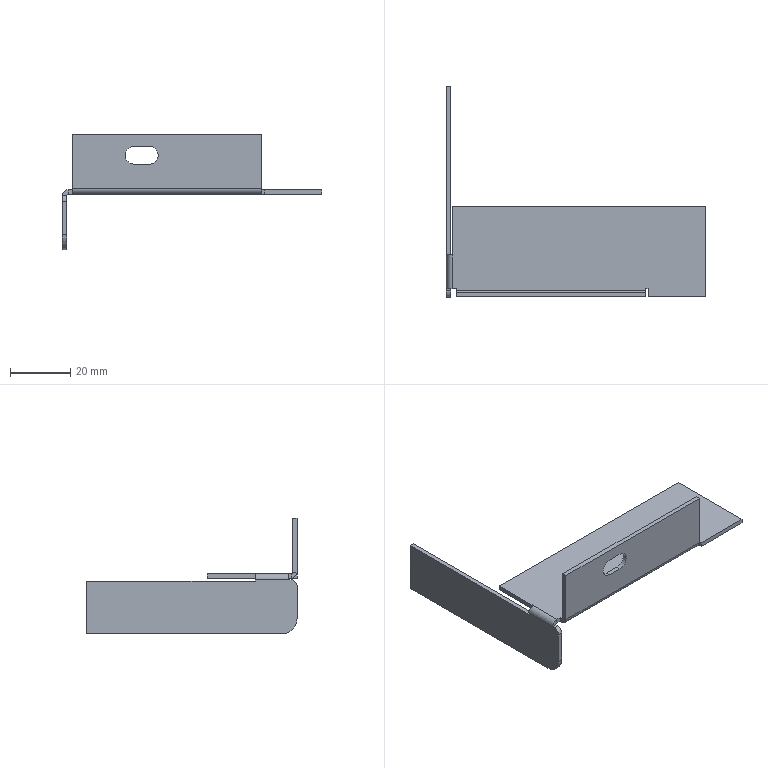Part | SolidWorks | features ICE 4, Fillet 2, EdgeFlange 1, FlatPattern 1, SMBaseFlange 1, SMMiteredFlange 1, SheetMetal 1 | 1 solid | 37 faces | box 86.5 x 70 x 38.5 mm | volume 7275 mm3 | plane 29 | cylinder 8 | commonest cylinder face diameters 4 x3 1 x2 6 x2 10 x1
STEP:
#1=CARTESIAN_POINT('',(-63.684,0.4966,0.));
#2=VERTEX_POINT('',#1);
#3=CARTESIAN_POINT('',(-63.684,-10.753,0.));
#4=VERTEX_POINT('',#3);
#5=CARTESIAN_POINT('',(-63.684,56.497,0.));
#6=DIRECTION('',(0.,-1.,0.));
#7=VECTOR('',#6,1000.);
#8=LINE('',#5,#7);
#9=EDGE_CURVE('',#2,#4,#8,.T.);
#10=ORIENTED_EDGE('',*,*,#9,.F.);
#11=CARTESIAN_POINT('',(-65.684,0.4966,-2.));
#12=VERTEX_POINT('',#11);
#13=CARTESIAN_POINT('',(-63.684,0.4966,-2.));
#14=DIRECTION('',(0.,-1.,0.));
#15=DIRECTION('',(0.,0.,1.));
#16=AXIS2_PLACEMENT_3D('',#13,#14,#15);
#17=CIRCLE('',#16,2.);
#18=EDGE_CURVE('',#2,#12,#17,.T.);
#19=ORIENTED_EDGE('',*,*,#18,.T.);
#20=CARTESIAN_POINT('',(-65.684,-10.753,-2.));
#21=VERTEX_POINT('',#20);
#22=CARTESIAN_POINT('',(-65.684,0.,-2.));
#23=DIRECTION('',(0.,1.,0.));
#24=VECTOR('',#23,1000.);
#25=LINE('',#22,#24);
#26=EDGE_CURVE('',#21,#12,#25,.T.);
#27=ORIENTED_EDGE('',*,*,#26,.F.);
#28=CARTESIAN_POINT('',(-63.684,-10.753,-2.));
#29=DIRECTION('',(0.,-1.,0.));
#30=DIRECTION('',(0.,0.,1.));
#31=AXIS2_PLACEMENT_3D('',#28,#29,#30);
#32=CIRCLE('',#31,2.);
#33=EDGE_CURVE('',#4,#21,#32,.T.);
#34=ORIENTED_EDGE('',*,*,#33,.F.);
#35=EDGE_LOOP('',(#10,#19,#27,#34));
#36=FACE_OUTER_BOUND('',#35,.T.);
#37=CARTESIAN_POINT('',(-63.684,56.497,-2.));
#38=DIRECTION('',(0.,1.,0.));
#39=DIRECTION('',(-1.,0.,0.));
#40=AXIS2_PLACEMENT_3D('',#37,#38,#39);
#41=CYLINDRICAL_SURFACE('',#40,2.);
#42=ADVANCED_FACE('',(#36),#41,.T.);
#43=CARTESIAN_POINT('',(-63.684,0.4966,-1.5));
#44=VERTEX_POINT('',#43);
#45=CARTESIAN_POINT('',(-64.184,0.4966,-2.));
#46=VERTEX_POINT('',#45);
#47=CARTESIAN_POINT('',(-63.684,0.4966,-2.));
#48=DIRECTION('',(0.,-1.,0.));
#49=DIRECTION('',(0.,0.,1.));
#50=AXIS2_PLACEMENT_3D('',#47,#48,#49);
#51=CIRCLE('',#50,0.5);
#52=EDGE_CURVE('',#44,#46,#51,.T.);
#53=ORIENTED_EDGE('',*,*,#52,.F.);
#54=CARTESIAN_POINT('',(-63.684,-10.753,-1.5));
#55=VERTEX_POINT('',#54);
#56=CARTESIAN_POINT('',(-63.684,56.497,-1.5));
#57=DIRECTION('',(0.,-1.,0.));
#58=VECTOR('',#57,1000.);
#59=LINE('',#56,#58);
#60=EDGE_CURVE('',#44,#55,#59,.T.);
#61=ORIENTED_EDGE('',*,*,#60,.T.);
#62=CARTESIAN_POINT('',(-64.184,-10.753,-2.));
#63=VERTEX_POINT('',#62);
#64=CARTESIAN_POINT('',(-63.684,-10.753,-2.));
#65=DIRECTION('',(0.,-1.,0.));
#66=DIRECTION('',(0.,0.,1.));
#67=AXIS2_PLACEMENT_3D('',#64,#65,#66);
#68=CIRCLE('',#67,0.5);
#69=EDGE_CURVE('',#55,#63,#68,.T.);
#70=ORIENTED_EDGE('',*,*,#69,.T.);
#71=CARTESIAN_POINT('',(-64.184,-13.503,-2.));
#72=DIRECTION('',(0.,1.,0.));
#73=VECTOR('',#72,1000.);
#74=LINE('',#71,#73);
#75=EDGE_CURVE('',#63,#46,#74,.T.);
#76=ORIENTED_EDGE('',*,*,#75,.T.);
#77=EDGE_LOOP('',(#53,#61,#70,#76));
#78=FACE_OUTER_BOUND('',#77,.T.);
#79=CARTESIAN_POINT('',(-63.684,56.497,-2.));
#80=DIRECTION('',(0.,1.,0.));
#81=DIRECTION('',(-1.,0.,0.));
#82=AXIS2_PLACEMENT_3D('',#79,#80,#81);
#83=CYLINDRICAL_SURFACE('',#82,0.5);
#84=ADVANCED_FACE('',(#78),#83,.F.);
#85=CARTESIAN_POINT('',(-62.184,-10.753,-1.5));
#86=VERTEX_POINT('',#85);
#87=CARTESIAN_POINT('',(-62.184,-10.753,-1.5));
#88=DIRECTION('',(-1.,0.,0.));
#89=VECTOR('',#88,1000.);
#90=LINE('',#87,#89);
#91=EDGE_CURVE('',#86,#55,#90,.T.);
#92=ORIENTED_EDGE('',*,*,#91,.T.);
#93=ORIENTED_EDGE('',*,*,#60,.F.);
#94=CARTESIAN_POINT('',(-63.684,16.497,-1.5));
#95=VERTEX_POINT('',#94);
#96=CARTESIAN_POINT('',(-63.684,56.497,-1.5));
#97=DIRECTION('',(0.,-1.,0.));
#98=VECTOR('',#97,1000.);
#99=LINE('',#96,#98);
#100=EDGE_CURVE('',#95,#44,#99,.T.);
#101=ORIENTED_EDGE('',*,*,#100,.F.);
#102=CARTESIAN_POINT('',(20.816,16.497,-1.5));
#103=VERTEX_POINT('',#102);
#104=CARTESIAN_POINT('',(0.,16.497,-1.5));
#105=DIRECTION('',(1.,0.,0.));
#106=VECTOR('',#105,1000.);
#107=LINE('',#104,#106);
#108=EDGE_CURVE('',#95,#103,#107,.T.);
#109=ORIENTED_EDGE('',*,*,#108,.T.);
#110=CARTESIAN_POINT('',(20.816,-13.503,-1.5));
#111=VERTEX_POINT('',#110);
#112=CARTESIAN_POINT('',(20.816,70.497,-1.5));
#113=DIRECTION('',(0.,1.,0.));
#114=VECTOR('',#113,1000.);
#115=LINE('',#112,#114);
#116=EDGE_CURVE('',#111,#103,#115,.T.);
#117=ORIENTED_EDGE('',*,*,#116,.F.);
#118=CARTESIAN_POINT('',(1.566,-13.503,-1.5));
#119=VERTEX_POINT('',#118);
#120=CARTESIAN_POINT('',(-64.184,-13.503,-1.5));
#121=DIRECTION('',(1.,0.,0.));
#122=VECTOR('',#121,1000.);
#123=LINE('',#120,#122);
#124=EDGE_CURVE('',#119,#111,#123,.T.);
#125=ORIENTED_EDGE('',*,*,#124,.F.);
#126=CARTESIAN_POINT('',(1.566,-10.753,-1.5));
#127=VERTEX_POINT('',#126);
#128=CARTESIAN_POINT('',(1.566,-10.753,-1.5));
#129=DIRECTION('',(0.,-1.,0.));
#130=VECTOR('',#129,1000.);
#131=LINE('',#128,#130);
#132=EDGE_CURVE('',#127,#119,#131,.T.);
#133=ORIENTED_EDGE('',*,*,#132,.F.);
#134=CARTESIAN_POINT('',(0.8165,-10.753,-1.5));
#135=VERTEX_POINT('',#134);
#136=CARTESIAN_POINT('',(0.8165,-10.753,-1.5));
#137=DIRECTION('',(1.,0.,0.));
#138=VECTOR('',#137,1000.);
#139=LINE('',#136,#138);
#140=EDGE_CURVE('',#135,#127,#139,.T.);
#141=ORIENTED_EDGE('',*,*,#140,.F.);
#142=CARTESIAN_POINT('',(0.8165,-11.503,-1.5));
#143=VERTEX_POINT('',#142);
#144=CARTESIAN_POINT('',(0.8165,-13.503,-1.5));
#145=DIRECTION('',(0.,1.,0.));
#146=VECTOR('',#145,1000.);
#147=LINE('',#144,#146);
#148=EDGE_CURVE('',#143,#135,#147,.T.);
#149=ORIENTED_EDGE('',*,*,#148,.F.);
#150=CARTESIAN_POINT('',(-62.184,-11.503,-1.5));
#151=VERTEX_POINT('',#150);
#152=CARTESIAN_POINT('',(445.816,-11.503,-1.5));
#153=DIRECTION('',(-1.,0.,0.));
#154=VECTOR('',#153,1000.);
#155=LINE('',#152,#154);
#156=EDGE_CURVE('',#143,#151,#155,.T.);
#157=ORIENTED_EDGE('',*,*,#156,.T.);
#158=CARTESIAN_POINT('',(-62.184,-13.503,-1.5));
#159=DIRECTION('',(0.,1.,0.));
#160=VECTOR('',#159,1000.);
#161=LINE('',#158,#160);
#162=EDGE_CURVE('',#151,#86,#161,.T.);
#163=ORIENTED_EDGE('',*,*,#162,.T.);
#164=EDGE_LOOP('',(#92,#93,#101,#109,#117,#125,#133,#141,#149,#157,#163));
#165=FACE_OUTER_BOUND('',#164,.T.);
#166=CARTESIAN_POINT('',(0.,0.,-1.5));
#167=DIRECTION('',(0.,0.,1.));
#168=DIRECTION('',(1.,0.,0.));
#169=AXIS2_PLACEMENT_3D('',#166,#167,#168);
#170=PLANE('',#169);
#171=ADVANCED_FACE('',(#165),#170,.F.);
#172=CARTESIAN_POINT('',(-63.684,16.497,0.));
#173=VERTEX_POINT('',#172);
#174=CARTESIAN_POINT('',(-63.684,56.497,0.));
#175=DIRECTION('',(0.,-1.,0.));
#176=VECTOR('',#175,1000.);
#177=LINE('',#174,#176);
#178=EDGE_CURVE('',#173,#2,#177,.T.);
#179=ORIENTED_EDGE('',*,*,#178,.T.);
#180=ORIENTED_EDGE('',*,*,#9,.T.);
#181=CARTESIAN_POINT('',(-62.184,-10.753,0.));
#182=VERTEX_POINT('',#181);
#183=CARTESIAN_POINT('',(-62.184,-10.753,0.));
#184=DIRECTION('',(-1.,0.,0.));
#185=VECTOR('',#184,1000.);
#186=LINE('',#183,#185);
#187=EDGE_CURVE('',#182,#4,#186,.T.);
#188=ORIENTED_EDGE('',*,*,#187,.F.);
#189=CARTESIAN_POINT('',(-62.184,-11.503,0.));
#190=VERTEX_POINT('',#189);
#191=CARTESIAN_POINT('',(-62.184,-13.503,0.));
#192=DIRECTION('',(0.,1.,0.));
#193=VECTOR('',#192,1000.);
#194=LINE('',#191,#193);
#195=EDGE_CURVE('',#190,#182,#194,.T.);
#196=ORIENTED_EDGE('',*,*,#195,.F.);
#197=CARTESIAN_POINT('',(0.8165,-11.503,0.));
#198=VERTEX_POINT('',#197);
#199=CARTESIAN_POINT('',(445.816,-11.503,0.));
#200=DIRECTION('',(-1.,0.,0.));
#201=VECTOR('',#200,1000.);
#202=LINE('',#199,#201);
#203=EDGE_CURVE('',#198,#190,#202,.T.);
#204=ORIENTED_EDGE('',*,*,#203,.F.);
#205=CARTESIAN_POINT('',(0.8165,-10.753,0.));
#206=VERTEX_POINT('',#205);
#207=CARTESIAN_POINT('',(0.8165,-13.503,0.));
#208=DIRECTION('',(0.,1.,0.));
#209=VECTOR('',#208,1000.);
#210=LINE('',#207,#209);
#211=EDGE_CURVE('',#198,#206,#210,.T.);
#212=ORIENTED_EDGE('',*,*,#211,.T.);
#213=CARTESIAN_POINT('',(1.566,-10.753,0.));
#214=VERTEX_POINT('',#213);
#215=CARTESIAN_POINT('',(0.8165,-10.753,0.));
#216=DIRECTION('',(1.,0.,0.));
#217=VECTOR('',#216,1000.);
#218=LINE('',#215,#217);
#219=EDGE_CURVE('',#206,#214,#218,.T.);
#220=ORIENTED_EDGE('',*,*,#219,.T.);
#221=CARTESIAN_POINT('',(1.566,-13.503,0.));
#222=VERTEX_POINT('',#221);
#223=CARTESIAN_POINT('',(1.566,-10.753,0.));
#224=DIRECTION('',(0.,-1.,0.));
#225=VECTOR('',#224,1000.);
#226=LINE('',#223,#225);
#227=EDGE_CURVE('',#214,#222,#226,.T.);
#228=ORIENTED_EDGE('',*,*,#227,.T.);
#229=CARTESIAN_POINT('',(20.816,-13.503,0.));
#230=VERTEX_POINT('',#229);
#231=CARTESIAN_POINT('',(-64.184,-13.503,0.));
#232=DIRECTION('',(1.,0.,0.));
#233=VECTOR('',#232,1000.);
#234=LINE('',#231,#233);
#235=EDGE_CURVE('',#222,#230,#234,.T.);
#236=ORIENTED_EDGE('',*,*,#235,.T.);
#237=CARTESIAN_POINT('',(20.816,16.497,0.));
#238=VERTEX_POINT('',#237);
#239=CARTESIAN_POINT('',(20.816,70.497,0.));
#240=DIRECTION('',(0.,1.,0.));
#241=VECTOR('',#240,1000.);
#242=LINE('',#239,#241);
#243=EDGE_CURVE('',#230,#238,#242,.T.);
#244=ORIENTED_EDGE('',*,*,#243,.T.);
#245=CARTESIAN_POINT('',(0.,16.497,0.));
#246=DIRECTION('',(1.,0.,0.));
#247=VECTOR('',#246,1000.);
#248=LINE('',#245,#247);
#249=EDGE_CURVE('',#173,#238,#248,.T.);
#250=ORIENTED_EDGE('',*,*,#249,.F.);
#251=EDGE_LOOP('',(#179,#180,#188,#196,#204,#212,#220,#228,#236,#244,#250));
#252=FACE_OUTER_BOUND('',#251,.T.);
#253=CARTESIAN_POINT('',(0.,0.,0.));
#254=DIRECTION('',(0.,0.,1.));
#255=DIRECTION('',(1.,0.,0.));
#256=AXIS2_PLACEMENT_3D('',#253,#254,#255);
#257=PLANE('',#256);
#258=ADVANCED_FACE('',(#252),#257,.T.);
#259=ORIENTED_EDGE('',*,*,#116,.T.);
#260=CARTESIAN_POINT('',(20.816,16.497,-1.5));
#261=DIRECTION('',(0.,0.,1.));
#262=VECTOR('',#261,1000.);
#263=LINE('',#260,#262);
#264=EDGE_CURVE('',#103,#238,#263,.T.);
#265=ORIENTED_EDGE('',*,*,#264,.T.);
#266=ORIENTED_EDGE('',*,*,#243,.F.);
#267=CARTESIAN_POINT('',(20.816,-13.503,-1.5));
#268=DIRECTION('',(0.,0.,1.));
#269=VECTOR('',#268,1000.);
#270=LINE('',#267,#269);
#271=EDGE_CURVE('',#111,#230,#270,.T.);
#272=ORIENTED_EDGE('',*,*,#271,.F.);
#273=EDGE_LOOP('',(#259,#265,#266,#272));
#274=FACE_OUTER_BOUND('',#273,.T.);
#275=CARTESIAN_POINT('',(20.816,70.497,-1.5));
#276=DIRECTION('',(1.,0.,0.));
#277=DIRECTION('',(0.,1.,0.));
#278=AXIS2_PLACEMENT_3D('',#275,#276,#277);
#279=PLANE('',#278);
#280=ADVANCED_FACE('',(#274),#279,.T.);
#281=CARTESIAN_POINT('',(1.566,-13.503,0.));
#282=DIRECTION('',(0.,0.,-1.));
#283=VECTOR('',#282,1000.);
#284=LINE('',#281,#283);
#285=EDGE_CURVE('',#222,#119,#284,.T.);
#286=ORIENTED_EDGE('',*,*,#285,.T.);
#287=ORIENTED_EDGE('',*,*,#124,.T.);
#288=ORIENTED_EDGE('',*,*,#271,.T.);
#289=ORIENTED_EDGE('',*,*,#235,.F.);
#290=EDGE_LOOP('',(#286,#287,#288,#289));
#291=FACE_OUTER_BOUND('',#290,.T.);
#292=CARTESIAN_POINT('',(-64.184,-13.503,-1.5));
#293=DIRECTION('',(0.,-1.,0.));
#294=DIRECTION('',(0.,0.,-1.));
#295=AXIS2_PLACEMENT_3D('',#292,#293,#294);
#296=PLANE('',#295);
#297=ADVANCED_FACE('',(#291),#296,.T.);
#298=CARTESIAN_POINT('',(0.8165,-11.503,-1.5));
#299=DIRECTION('',(0.,0.,1.));
#300=VECTOR('',#299,1000.);
#301=LINE('',#298,#300);
#302=EDGE_CURVE('',#143,#198,#301,.T.);
#303=ORIENTED_EDGE('',*,*,#302,.F.);
#304=ORIENTED_EDGE('',*,*,#148,.T.);
#305=CARTESIAN_POINT('',(0.8165,-10.753,0.));
#306=DIRECTION('',(0.,0.,-1.));
#307=VECTOR('',#306,1000.);
#308=LINE('',#305,#307);
#309=EDGE_CURVE('',#206,#135,#308,.T.);
#310=ORIENTED_EDGE('',*,*,#309,.F.);
#311=ORIENTED_EDGE('',*,*,#211,.F.);
#312=EDGE_LOOP('',(#303,#304,#310,#311));
#313=FACE_OUTER_BOUND('',#312,.T.);
#314=CARTESIAN_POINT('',(0.8165,-13.503,0.));
#315=DIRECTION('',(-1.,0.,0.));
#316=DIRECTION('',(0.,0.,1.));
#317=AXIS2_PLACEMENT_3D('',#314,#315,#316);
#318=PLANE('',#317);
#319=ADVANCED_FACE('',(#313),#318,.F.);
#320=ORIENTED_EDGE('',*,*,#140,.T.);
#321=CARTESIAN_POINT('',(1.566,-10.753,0.));
#322=DIRECTION('',(0.,0.,-1.));
#323=VECTOR('',#322,1000.);
#324=LINE('',#321,#323);
#325=EDGE_CURVE('',#214,#127,#324,.T.);
#326=ORIENTED_EDGE('',*,*,#325,.F.);
#327=ORIENTED_EDGE('',*,*,#219,.F.);
#328=ORIENTED_EDGE('',*,*,#309,.T.);
#329=EDGE_LOOP('',(#320,#326,#327,#328));
#330=FACE_OUTER_BOUND('',#329,.T.);
#331=CARTESIAN_POINT('',(0.8165,-10.753,0.));
#332=DIRECTION('',(0.,1.,0.));
#333=DIRECTION('',(0.,0.,1.));
#334=AXIS2_PLACEMENT_3D('',#331,#332,#333);
#335=PLANE('',#334);
#336=ADVANCED_FACE('',(#330),#335,.F.);
#337=ORIENTED_EDGE('',*,*,#132,.T.);
#338=ORIENTED_EDGE('',*,*,#285,.F.);
#339=ORIENTED_EDGE('',*,*,#227,.F.);
#340=ORIENTED_EDGE('',*,*,#325,.T.);
#341=EDGE_LOOP('',(#337,#338,#339,#340));
#342=FACE_OUTER_BOUND('',#341,.T.);
#343=CARTESIAN_POINT('',(1.566,-10.753,0.));
#344=DIRECTION('',(1.,0.,0.));
#345=DIRECTION('',(0.,0.,-1.));
#346=AXIS2_PLACEMENT_3D('',#343,#344,#345);
#347=PLANE('',#346);
#348=ADVANCED_FACE('',(#342),#347,.F.);
#349=ORIENTED_EDGE('',*,*,#195,.T.);
#350=CARTESIAN_POINT('',(-62.184,-10.753,0.));
#351=DIRECTION('',(0.,0.,-1.));
#352=VECTOR('',#351,1000.);
#353=LINE('',#350,#352);
#354=EDGE_CURVE('',#182,#86,#353,.T.);
#355=ORIENTED_EDGE('',*,*,#354,.T.);
#356=ORIENTED_EDGE('',*,*,#162,.F.);
#357=CARTESIAN_POINT('',(-62.184,-11.503,-1.5));
#358=DIRECTION('',(0.,0.,1.));
#359=VECTOR('',#358,1000.);
#360=LINE('',#357,#359);
#361=EDGE_CURVE('',#151,#190,#360,.T.);
#362=ORIENTED_EDGE('',*,*,#361,.T.);
#363=EDGE_LOOP('',(#349,#355,#356,#362));
#364=FACE_OUTER_BOUND('',#363,.T.);
#365=CARTESIAN_POINT('',(-62.184,-13.503,0.));
#366=DIRECTION('',(-1.,0.,0.));
#367=DIRECTION('',(0.,0.,1.));
#368=AXIS2_PLACEMENT_3D('',#365,#366,#367);
#369=PLANE('',#368);
#370=ADVANCED_FACE('',(#364),#369,.T.);
#371=ORIENTED_EDGE('',*,*,#91,.F.);
#372=ORIENTED_EDGE('',*,*,#354,.F.);
#373=ORIENTED_EDGE('',*,*,#187,.T.);
#374=CARTESIAN_POINT('',(-63.684,-10.753,0.));
#375=DIRECTION('',(0.,0.,-1.));
#376=VECTOR('',#375,1000.);
#377=LINE('',#374,#376);
#378=EDGE_CURVE('',#4,#55,#377,.T.);
#379=ORIENTED_EDGE('',*,*,#378,.T.);
#380=EDGE_LOOP('',(#371,#372,#373,#379));
#381=FACE_OUTER_BOUND('',#380,.T.);
#382=CARTESIAN_POINT('',(-62.184,-10.753,0.));
#383=DIRECTION('',(0.,-1.,0.));
#384=DIRECTION('',(0.,0.,-1.));
#385=AXIS2_PLACEMENT_3D('',#382,#383,#384);
#386=PLANE('',#385);
#387=ADVANCED_FACE('',(#381),#386,.T.);
#388=CARTESIAN_POINT('',(-62.184,-13.503,18.5));
#389=VERTEX_POINT('',#388);
#390=CARTESIAN_POINT('',(-62.184,-12.003,18.5));
#391=VERTEX_POINT('',#390);
#392=CARTESIAN_POINT('',(-62.184,-13.503,18.5));
#393=DIRECTION('',(0.,1.,0.));
#394=VECTOR('',#393,1000.);
#395=LINE('',#392,#394);
#396=EDGE_CURVE('',#389,#391,#395,.T.);
#397=ORIENTED_EDGE('',*,*,#396,.F.);
#398=CARTESIAN_POINT('',(0.8165,-13.503,18.5));
#399=VERTEX_POINT('',#398);
#400=CARTESIAN_POINT('',(20.816,-13.503,18.5));
#401=DIRECTION('',(-1.,0.,0.));
#402=VECTOR('',#401,1000.);
#403=LINE('',#400,#402);
#404=EDGE_CURVE('',#399,#389,#403,.T.);
#405=ORIENTED_EDGE('',*,*,#404,.F.);
#406=CARTESIAN_POINT('',(0.8165,-12.003,18.5));
#407=VERTEX_POINT('',#406);
#408=CARTESIAN_POINT('',(0.8165,-13.503,18.5));
#409=DIRECTION('',(0.,1.,0.));
#410=VECTOR('',#409,1000.);
#411=LINE('',#408,#410);
#412=EDGE_CURVE('',#399,#407,#411,.T.);
#413=ORIENTED_EDGE('',*,*,#412,.T.);
#414=CARTESIAN_POINT('',(20.816,-12.003,18.5));
#415=DIRECTION('',(-1.,0.,0.));
#416=VECTOR('',#415,1000.);
#417=LINE('',#414,#416);
#418=EDGE_CURVE('',#407,#391,#417,.T.);
#419=ORIENTED_EDGE('',*,*,#418,.T.);
#420=EDGE_LOOP('',(#397,#405,#413,#419));
#421=FACE_OUTER_BOUND('',#420,.T.);
#422=CARTESIAN_POINT('',(20.816,-13.503,18.5));
#423=DIRECTION('',(0.,0.,-1.));
#424=DIRECTION('',(-1.,0.,0.));
#425=AXIS2_PLACEMENT_3D('',#422,#423,#424);
#426=PLANE('',#425);
#427=ADVANCED_FACE('',(#421),#426,.F.);
#428=ORIENTED_EDGE('',*,*,#412,.F.);
#429=CARTESIAN_POINT('',(0.8165,-13.503,0.5));
#430=VERTEX_POINT('',#429);
#431=CARTESIAN_POINT('',(0.8165,-13.503,18.5));
#432=DIRECTION('',(0.,0.,-1.));
#433=VECTOR('',#432,1000.);
#434=LINE('',#431,#433);
#435=EDGE_CURVE('',#399,#430,#434,.T.);
#436=ORIENTED_EDGE('',*,*,#435,.T.);
#437=CARTESIAN_POINT('',(0.8165,-12.003,0.5));
#438=VERTEX_POINT('',#437);
#439=CARTESIAN_POINT('',(0.8165,-13.503,0.5));
#440=DIRECTION('',(0.,1.,0.));
#441=VECTOR('',#440,1000.);
#442=LINE('',#439,#441);
#443=EDGE_CURVE('',#430,#438,#442,.T.);
#444=ORIENTED_EDGE('',*,*,#443,.T.);
#445=CARTESIAN_POINT('',(0.8165,-12.003,18.5));
#446=DIRECTION('',(0.,0.,-1.));
#447=VECTOR('',#446,1000.);
#448=LINE('',#445,#447);
#449=EDGE_CURVE('',#407,#438,#448,.T.);
#450=ORIENTED_EDGE('',*,*,#449,.F.);
#451=EDGE_LOOP('',(#428,#436,#444,#450));
#452=FACE_OUTER_BOUND('',#451,.T.);
#453=CARTESIAN_POINT('',(0.8165,-13.503,18.5));
#454=DIRECTION('',(1.,0.,0.));
#455=DIRECTION('',(0.,0.,-1.));
#456=AXIS2_PLACEMENT_3D('',#453,#454,#455);
#457=PLANE('',#456);
#458=ADVANCED_FACE('',(#452),#457,.T.);
#459=CARTESIAN_POINT('',(-62.184,-13.503,0.5));
#460=VERTEX_POINT('',#459);
#461=CARTESIAN_POINT('',(-62.184,-13.503,18.5));
#462=DIRECTION('',(0.,0.,1.));
#463=VECTOR('',#462,1000.);
#464=LINE('',#461,#463);
#465=EDGE_CURVE('',#460,#389,#464,.T.);
#466=ORIENTED_EDGE('',*,*,#465,.T.);
#467=ORIENTED_EDGE('',*,*,#396,.T.);
#468=CARTESIAN_POINT('',(-62.184,-12.003,0.5));
#469=VERTEX_POINT('',#468);
#470=CARTESIAN_POINT('',(-62.184,-12.003,18.5));
#471=DIRECTION('',(0.,0.,1.));
#472=VECTOR('',#471,1000.);
#473=LINE('',#470,#472);
#474=EDGE_CURVE('',#469,#391,#473,.T.);
#475=ORIENTED_EDGE('',*,*,#474,.F.);
#476=CARTESIAN_POINT('',(-62.184,-13.503,0.5));
#477=DIRECTION('',(0.,1.,0.));
#478=VECTOR('',#477,1000.);
#479=LINE('',#476,#478);
#480=EDGE_CURVE('',#460,#469,#479,.T.);
#481=ORIENTED_EDGE('',*,*,#480,.F.);
#482=EDGE_LOOP('',(#466,#467,#475,#481));
#483=FACE_OUTER_BOUND('',#482,.T.);
#484=CARTESIAN_POINT('',(-62.184,-13.503,18.5));
#485=DIRECTION('',(-1.,0.,0.));
#486=DIRECTION('',(0.,0.,1.));
#487=AXIS2_PLACEMENT_3D('',#484,#485,#486);
#488=PLANE('',#487);
#489=ADVANCED_FACE('',(#483),#488,.T.);
#490=CARTESIAN_POINT('',(-41.684,-12.003,8.5));
#491=VERTEX_POINT('',#490);
#492=CARTESIAN_POINT('',(-41.684,-12.003,14.5));
#493=VERTEX_POINT('',#492);
#494=CARTESIAN_POINT('',(-41.684,-12.003,11.5));
#495=DIRECTION('',(0.,1.,0.));
#496=DIRECTION('',(0.,0.,1.));
#497=AXIS2_PLACEMENT_3D('',#494,#495,#496);
#498=CIRCLE('',#497,3.);
#499=EDGE_CURVE('',#491,#493,#498,.T.);
#500=ORIENTED_EDGE('',*,*,#499,.F.);
#501=CARTESIAN_POINT('',(-36.684,-12.003,8.5));
#502=VERTEX_POINT('',#501);
#503=CARTESIAN_POINT('',(-41.684,-12.003,8.5));
#504=DIRECTION('',(-1.,0.,0.));
#505=VECTOR('',#504,1000.);
#506=LINE('',#503,#505);
#507=EDGE_CURVE('',#502,#491,#506,.T.);
#508=ORIENTED_EDGE('',*,*,#507,.F.);
#509=CARTESIAN_POINT('',(-36.684,-12.003,14.5));
#510=VERTEX_POINT('',#509);
#511=CARTESIAN_POINT('',(-36.684,-12.003,11.5));
#512=DIRECTION('',(0.,1.,0.));
#513=DIRECTION('',(0.,0.,1.));
#514=AXIS2_PLACEMENT_3D('',#511,#512,#513);
#515=CIRCLE('',#514,3.);
#516=EDGE_CURVE('',#510,#502,#515,.T.);
#517=ORIENTED_EDGE('',*,*,#516,.F.);
#518=CARTESIAN_POINT('',(-41.684,-12.003,14.5));
#519=DIRECTION('',(1.,0.,0.));
#520=VECTOR('',#519,1000.);
#521=LINE('',#518,#520);
#522=EDGE_CURVE('',#493,#510,#521,.T.);
#523=ORIENTED_EDGE('',*,*,#522,.F.);
#524=EDGE_LOOP('',(#500,#508,#517,#523));
#525=FACE_BOUND('',#524,.T.);
#526=CARTESIAN_POINT('',(20.816,-12.003,0.5));
#527=DIRECTION('',(-1.,0.,0.));
#528=VECTOR('',#527,1000.);
#529=LINE('',#526,#528);
#530=EDGE_CURVE('',#438,#469,#529,.T.);
#531=ORIENTED_EDGE('',*,*,#530,.T.);
#532=ORIENTED_EDGE('',*,*,#474,.T.);
#533=ORIENTED_EDGE('',*,*,#418,.F.);
#534=ORIENTED_EDGE('',*,*,#449,.T.);
#535=EDGE_LOOP('',(#531,#532,#533,#534));
#536=FACE_OUTER_BOUND('',#535,.T.);
#537=CARTESIAN_POINT('',(20.816,-12.003,18.5));
#538=DIRECTION('',(0.,1.,0.));
#539=DIRECTION('',(0.,0.,1.));
#540=AXIS2_PLACEMENT_3D('',#537,#538,#539);
#541=PLANE('',#540);
#542=ADVANCED_FACE('',(#525,#536),#541,.T.);
#543=CARTESIAN_POINT('',(-36.684,-13.503,8.5));
#544=VERTEX_POINT('',#543);
#545=CARTESIAN_POINT('',(-41.684,-13.503,8.5));
#546=VERTEX_POINT('',#545);
#547=CARTESIAN_POINT('',(20.816,-13.503,8.5));
#548=DIRECTION('',(-1.,0.,0.));
#549=VECTOR('',#548,1000.);
#550=LINE('',#547,#549);
#551=EDGE_CURVE('',#544,#546,#550,.T.);
#552=ORIENTED_EDGE('',*,*,#551,.T.);
#553=CARTESIAN_POINT('',(-41.684,-13.503,14.5));
#554=VERTEX_POINT('',#553);
#555=CARTESIAN_POINT('',(-41.684,-13.503,11.5));
#556=DIRECTION('',(0.,1.,0.));
#557=DIRECTION('',(0.,0.,1.));
#558=AXIS2_PLACEMENT_3D('',#555,#556,#557);
#559=CIRCLE('',#558,3.);
#560=EDGE_CURVE('',#546,#554,#559,.T.);
#561=ORIENTED_EDGE('',*,*,#560,.T.);
#562=CARTESIAN_POINT('',(-36.684,-13.503,14.5));
#563=VERTEX_POINT('',#562);
#564=CARTESIAN_POINT('',(20.816,-13.503,14.5));
#565=DIRECTION('',(1.,0.,0.));
#566=VECTOR('',#565,1000.);
#567=LINE('',#564,#566);
#568=EDGE_CURVE('',#554,#563,#567,.T.);
#569=ORIENTED_EDGE('',*,*,#568,.T.);
#570=CARTESIAN_POINT('',(-36.684,-13.503,11.5));
#571=DIRECTION('',(0.,1.,0.));
#572=DIRECTION('',(0.,0.,1.));
#573=AXIS2_PLACEMENT_3D('',#570,#571,#572);
#574=CIRCLE('',#573,3.);
#575=EDGE_CURVE('',#563,#544,#574,.T.);
#576=ORIENTED_EDGE('',*,*,#575,.T.);
#577=EDGE_LOOP('',(#552,#561,#569,#576));
#578=FACE_BOUND('',#577,.T.);
#579=CARTESIAN_POINT('',(20.816,-13.503,0.5));
#580=DIRECTION('',(-1.,0.,0.));
#581=VECTOR('',#580,1000.);
#582=LINE('',#579,#581);
#583=EDGE_CURVE('',#430,#460,#582,.T.);
#584=ORIENTED_EDGE('',*,*,#583,.F.);
#585=ORIENTED_EDGE('',*,*,#435,.F.);
#586=ORIENTED_EDGE('',*,*,#404,.T.);
#587=ORIENTED_EDGE('',*,*,#465,.F.);
#588=EDGE_LOOP('',(#584,#585,#586,#587));
#589=FACE_OUTER_BOUND('',#588,.T.);
#590=CARTESIAN_POINT('',(20.816,-13.503,18.5));
#591=DIRECTION('',(0.,1.,0.));
#592=DIRECTION('',(0.,0.,1.));
#593=AXIS2_PLACEMENT_3D('',#590,#591,#592);
#594=PLANE('',#593);
#595=ADVANCED_FACE('',(#578,#589),#594,.F.);
#596=ORIENTED_EDGE('',*,*,#443,.F.);
#597=CARTESIAN_POINT('',(0.8165,-11.503,0.5));
#598=DIRECTION('',(1.,0.,0.));
#599=DIRECTION('',(0.,0.,-1.));
#600=AXIS2_PLACEMENT_3D('',#597,#598,#599);
#601=CIRCLE('',#600,2.);
#602=EDGE_CURVE('',#430,#143,#601,.T.);
#603=ORIENTED_EDGE('',*,*,#602,.T.);
#604=ORIENTED_EDGE('',*,*,#302,.T.);
#605=CARTESIAN_POINT('',(0.8165,-11.503,0.5));
#606=DIRECTION('',(1.,0.,0.));
#607=DIRECTION('',(0.,0.,1.));
#608=AXIS2_PLACEMENT_3D('',#605,#606,#607);
#609=CIRCLE('',#608,0.5);
#610=EDGE_CURVE('',#438,#198,#609,.T.);
#611=ORIENTED_EDGE('',*,*,#610,.F.);
#612=EDGE_LOOP('',(#596,#603,#604,#611));
#613=FACE_OUTER_BOUND('',#612,.T.);
#614=CARTESIAN_POINT('',(0.8165,-11.503,0.5));
#615=DIRECTION('',(-1.,0.,0.));
#616=DIRECTION('',(0.,0.,1.));
#617=AXIS2_PLACEMENT_3D('',#614,#615,#616);
#618=PLANE('',#617);
#619=ADVANCED_FACE('',(#613),#618,.F.);
#620=CARTESIAN_POINT('',(-62.184,-11.503,0.5));
#621=DIRECTION('',(-1.,0.,0.));
#622=DIRECTION('',(0.,0.,1.));
#623=AXIS2_PLACEMENT_3D('',#620,#621,#622);
#624=CIRCLE('',#623,2.);
#625=EDGE_CURVE('',#151,#460,#624,.T.);
#626=ORIENTED_EDGE('',*,*,#625,.T.);
#627=ORIENTED_EDGE('',*,*,#480,.T.);
#628=CARTESIAN_POINT('',(-62.184,-11.503,0.5));
#629=DIRECTION('',(-1.,0.,0.));
#630=DIRECTION('',(0.,0.,1.));
#631=AXIS2_PLACEMENT_3D('',#628,#629,#630);
#632=CIRCLE('',#631,0.5);
#633=EDGE_CURVE('',#190,#469,#632,.T.);
#634=ORIENTED_EDGE('',*,*,#633,.F.);
#635=ORIENTED_EDGE('',*,*,#361,.F.);
#636=EDGE_LOOP('',(#626,#627,#634,#635));
#637=FACE_OUTER_BOUND('',#636,.T.);
#638=CARTESIAN_POINT('',(-62.184,-11.503,0.5));
#639=DIRECTION('',(1.,0.,0.));
#640=DIRECTION('',(0.,0.,-1.));
#641=AXIS2_PLACEMENT_3D('',#638,#639,#640);
#642=PLANE('',#641);
#643=ADVANCED_FACE('',(#637),#642,.F.);
#644=ORIENTED_EDGE('',*,*,#203,.T.);
#645=ORIENTED_EDGE('',*,*,#633,.T.);
#646=ORIENTED_EDGE('',*,*,#530,.F.);
#647=ORIENTED_EDGE('',*,*,#610,.T.);
#648=EDGE_LOOP('',(#644,#645,#646,#647));
#649=FACE_OUTER_BOUND('',#648,.T.);
#650=CARTESIAN_POINT('',(445.816,-11.503,0.5));
#651=DIRECTION('',(-1.,0.,0.));
#652=DIRECTION('',(0.,0.,1.));
#653=AXIS2_PLACEMENT_3D('',#650,#651,#652);
#654=CYLINDRICAL_SURFACE('',#653,0.5);
#655=ADVANCED_FACE('',(#649),#654,.F.);
#656=ORIENTED_EDGE('',*,*,#156,.F.);
#657=ORIENTED_EDGE('',*,*,#602,.F.);
#658=ORIENTED_EDGE('',*,*,#583,.T.);
#659=ORIENTED_EDGE('',*,*,#625,.F.);
#660=EDGE_LOOP('',(#656,#657,#658,#659));
#661=FACE_OUTER_BOUND('',#660,.T.);
#662=CARTESIAN_POINT('',(445.816,-11.503,0.5));
#663=DIRECTION('',(-1.,0.,0.));
#664=DIRECTION('',(0.,0.,1.));
#665=AXIS2_PLACEMENT_3D('',#662,#663,#664);
#666=CYLINDRICAL_SURFACE('',#665,2.);
#667=ADVANCED_FACE('',(#661),#666,.T.);
#668=CARTESIAN_POINT('',(-64.184,56.497,-2.5));
#669=VERTEX_POINT('',#668);
#670=CARTESIAN_POINT('',(-65.684,56.497,-2.5));
#671=VERTEX_POINT('',#670);
#672=CARTESIAN_POINT('',(-63.684,56.497,-2.5));
#673=DIRECTION('',(-1.,0.,0.));
#674=VECTOR('',#673,1000.);
#675=LINE('',#672,#674);
#676=EDGE_CURVE('',#669,#671,#675,.T.);
#677=ORIENTED_EDGE('',*,*,#676,.F.);
#678=CARTESIAN_POINT('',(-64.184,56.497,-20.));
#679=VERTEX_POINT('',#678);
#680=CARTESIAN_POINT('',(-64.184,56.497,-1.5));
#681=DIRECTION('',(0.,0.,1.));
#682=VECTOR('',#681,1000.);
#683=LINE('',#680,#682);
#684=EDGE_CURVE('',#679,#669,#683,.T.);
#685=ORIENTED_EDGE('',*,*,#684,.F.);
#686=CARTESIAN_POINT('',(-65.684,56.497,-20.));
#687=VERTEX_POINT('',#686);
#688=CARTESIAN_POINT('',(-65.684,56.497,-20.));
#689=DIRECTION('',(1.,0.,0.));
#690=VECTOR('',#689,1000.);
#691=LINE('',#688,#690);
#692=EDGE_CURVE('',#687,#679,#691,.T.);
#693=ORIENTED_EDGE('',*,*,#692,.F.);
#694=CARTESIAN_POINT('',(-65.684,56.497,-1.5));
#695=DIRECTION('',(0.,0.,1.));
#696=VECTOR('',#695,1000.);
#697=LINE('',#694,#696);
#698=EDGE_CURVE('',#687,#671,#697,.T.);
#699=ORIENTED_EDGE('',*,*,#698,.T.);
#700=EDGE_LOOP('',(#677,#685,#693,#699));
#701=FACE_OUTER_BOUND('',#700,.T.);
#702=CARTESIAN_POINT('',(-65.684,56.497,-1.5));
#703=DIRECTION('',(0.,1.,0.));
#704=DIRECTION('',(0.,0.,1.));
#705=AXIS2_PLACEMENT_3D('',#702,#703,#704);
#706=PLANE('',#705);
#707=ADVANCED_FACE('',(#701),#706,.T.);
#708=CARTESIAN_POINT('',(-64.184,-13.503,-4.));
#709=VERTEX_POINT('',#708);
#710=CARTESIAN_POINT('',(-64.184,-13.503,-15.));
#711=VERTEX_POINT('',#710);
#712=CARTESIAN_POINT('',(-64.184,-13.503,-20.));
#713=DIRECTION('',(0.,0.,-1.));
#714=VECTOR('',#713,1000.);
#715=LINE('',#712,#714);
#716=EDGE_CURVE('',#709,#711,#715,.T.);
#717=ORIENTED_EDGE('',*,*,#716,.F.);
#718=CARTESIAN_POINT('',(-65.684,-13.503,-4.));
#719=VERTEX_POINT('',#718);
#720=CARTESIAN_POINT('',(-65.684,-13.503,-4.));
#721=DIRECTION('',(-1.,0.,0.));
#722=VECTOR('',#721,1000.);
#723=LINE('',#720,#722);
#724=EDGE_CURVE('',#709,#719,#723,.T.);
#725=ORIENTED_EDGE('',*,*,#724,.T.);
#726=CARTESIAN_POINT('',(-65.684,-13.503,-15.));
#727=VERTEX_POINT('',#726);
#728=CARTESIAN_POINT('',(-65.684,-13.503,-20.));
#729=DIRECTION('',(0.,0.,-1.));
#730=VECTOR('',#729,1000.);
#731=LINE('',#728,#730);
#732=EDGE_CURVE('',#719,#727,#731,.T.);
#733=ORIENTED_EDGE('',*,*,#732,.T.);
#734=CARTESIAN_POINT('',(-65.684,-13.503,-15.));
#735=DIRECTION('',(1.,0.,0.));
#736=VECTOR('',#735,1000.);
#737=LINE('',#734,#736);
#738=EDGE_CURVE('',#727,#711,#737,.T.);
#739=ORIENTED_EDGE('',*,*,#738,.T.);
#740=EDGE_LOOP('',(#717,#725,#733,#739));
#741=FACE_OUTER_BOUND('',#740,.T.);
#742=CARTESIAN_POINT('',(-65.684,-13.503,-20.));
#743=DIRECTION('',(0.,-1.,0.));
#744=DIRECTION('',(1.,0.,0.));
#745=AXIS2_PLACEMENT_3D('',#742,#743,#744);
#746=PLANE('',#745);
#747=ADVANCED_FACE('',(#741),#746,.T.);
#748=ORIENTED_EDGE('',*,*,#732,.F.);
#749=CARTESIAN_POINT('',(-65.684,-11.503,-2.));
#750=VERTEX_POINT('',#749);
#751=CARTESIAN_POINT('',(-65.684,-11.503,-4.));
#752=DIRECTION('',(-1.,0.,0.));
#753=DIRECTION('',(0.,0.,1.));
#754=AXIS2_PLACEMENT_3D('',#751,#752,#753);
#755=CIRCLE('',#754,2.);
#756=EDGE_CURVE('',#719,#750,#755,.T.);
#757=ORIENTED_EDGE('',*,*,#756,.T.);
#758=CARTESIAN_POINT('',(-65.684,0.,-2.));
#759=DIRECTION('',(0.,1.,0.));
#760=VECTOR('',#759,1000.);
#761=LINE('',#758,#760);
#762=EDGE_CURVE('',#750,#21,#761,.T.);
#763=ORIENTED_EDGE('',*,*,#762,.T.);
#764=ORIENTED_EDGE('',*,*,#26,.T.);
#765=CARTESIAN_POINT('',(-65.684,0.4966,-2.5));
#766=VERTEX_POINT('',#765);
#767=CARTESIAN_POINT('',(-65.684,0.4966,0.));
#768=DIRECTION('',(0.,0.,-1.));
#769=VECTOR('',#768,1000.);
#770=LINE('',#767,#769);
#771=EDGE_CURVE('',#12,#766,#770,.T.);
#772=ORIENTED_EDGE('',*,*,#771,.T.);
#773=CARTESIAN_POINT('',(-65.684,0.,-2.5));
#774=DIRECTION('',(0.,-1.,0.));
#775=VECTOR('',#774,1000.);
#776=LINE('',#773,#775);
#777=EDGE_CURVE('',#671,#766,#776,.T.);
#778=ORIENTED_EDGE('',*,*,#777,.F.);
#779=ORIENTED_EDGE('',*,*,#698,.F.);
#780=CARTESIAN_POINT('',(-65.684,-8.503,-20.));
#781=VERTEX_POINT('',#780);
#782=CARTESIAN_POINT('',(-65.684,56.497,-20.));
#783=DIRECTION('',(0.,1.,0.));
#784=VECTOR('',#783,1000.);
#785=LINE('',#782,#784);
#786=EDGE_CURVE('',#781,#687,#785,.T.);
#787=ORIENTED_EDGE('',*,*,#786,.F.);
#788=CARTESIAN_POINT('',(-65.684,-8.503,-15.));
#789=DIRECTION('',(-1.,0.,0.));
#790=DIRECTION('',(0.,0.,1.));
#791=AXIS2_PLACEMENT_3D('',#788,#789,#790);
#792=CIRCLE('',#791,5.);
#793=EDGE_CURVE('',#781,#727,#792,.T.);
#794=ORIENTED_EDGE('',*,*,#793,.T.);
#795=EDGE_LOOP('',(#748,#757,#763,#764,#772,#778,#779,#787,#794));
#796=FACE_OUTER_BOUND('',#795,.T.);
#797=CARTESIAN_POINT('',(-65.684,0.,0.));
#798=DIRECTION('',(-1.,0.,0.));
#799=DIRECTION('',(0.,0.,1.));
#800=AXIS2_PLACEMENT_3D('',#797,#798,#799);
#801=PLANE('',#800);
#802=ADVANCED_FACE('',(#796),#801,.T.);
#803=CARTESIAN_POINT('',(-64.184,-11.503,-2.));
#804=VERTEX_POINT('',#803);
#805=CARTESIAN_POINT('',(-64.184,-13.503,-2.));
#806=DIRECTION('',(0.,1.,0.));
#807=VECTOR('',#806,1000.);
#808=LINE('',#805,#807);
#809=EDGE_CURVE('',#804,#63,#808,.T.);
#810=ORIENTED_EDGE('',*,*,#809,.F.);
#811=CARTESIAN_POINT('',(-64.184,-11.503,-4.));
#812=DIRECTION('',(1.,0.,0.));
#813=DIRECTION('',(0.,0.,1.));
#814=AXIS2_PLACEMENT_3D('',#811,#812,#813);
#815=CIRCLE('',#814,2.);
#816=EDGE_CURVE('',#804,#709,#815,.T.);
#817=ORIENTED_EDGE('',*,*,#816,.T.);
#818=ORIENTED_EDGE('',*,*,#716,.T.);
#819=CARTESIAN_POINT('',(-64.184,-8.503,-20.));
#820=VERTEX_POINT('',#819);
#821=CARTESIAN_POINT('',(-64.184,-8.503,-15.));
#822=DIRECTION('',(1.,0.,0.));
#823=DIRECTION('',(0.,0.,1.));
#824=AXIS2_PLACEMENT_3D('',#821,#822,#823);
#825=CIRCLE('',#824,5.);
#826=EDGE_CURVE('',#711,#820,#825,.T.);
#827=ORIENTED_EDGE('',*,*,#826,.T.);
#828=CARTESIAN_POINT('',(-64.184,56.497,-20.));
#829=DIRECTION('',(0.,1.,0.));
#830=VECTOR('',#829,1000.);
#831=LINE('',#828,#830);
#832=EDGE_CURVE('',#820,#679,#831,.T.);
#833=ORIENTED_EDGE('',*,*,#832,.T.);
#834=ORIENTED_EDGE('',*,*,#684,.T.);
#835=CARTESIAN_POINT('',(-64.184,0.4966,-2.5));
#836=VERTEX_POINT('',#835);
#837=CARTESIAN_POINT('',(-64.184,0.,-2.5));
#838=DIRECTION('',(0.,-1.,0.));
#839=VECTOR('',#838,1000.);
#840=LINE('',#837,#839);
#841=EDGE_CURVE('',#669,#836,#840,.T.);
#842=ORIENTED_EDGE('',*,*,#841,.T.);
#843=CARTESIAN_POINT('',(-64.184,0.4966,0.));
#844=DIRECTION('',(0.,0.,-1.));
#845=VECTOR('',#844,1000.);
#846=LINE('',#843,#845);
#847=EDGE_CURVE('',#46,#836,#846,.T.);
#848=ORIENTED_EDGE('',*,*,#847,.F.);
#849=ORIENTED_EDGE('',*,*,#75,.F.);
#850=EDGE_LOOP('',(#810,#817,#818,#827,#833,#834,#842,#848,#849));
#851=FACE_OUTER_BOUND('',#850,.T.);
#852=CARTESIAN_POINT('',(-64.184,0.,0.));
#853=DIRECTION('',(-1.,0.,0.));
#854=DIRECTION('',(0.,0.,1.));
#855=AXIS2_PLACEMENT_3D('',#852,#853,#854);
#856=PLANE('',#855);
#857=ADVANCED_FACE('',(#851),#856,.F.);
#858=ORIENTED_EDGE('',*,*,#832,.F.);
#859=CARTESIAN_POINT('',(-65.684,-8.503,-20.));
#860=DIRECTION('',(-1.,0.,0.));
#861=VECTOR('',#860,1000.);
#862=LINE('',#859,#861);
#863=EDGE_CURVE('',#820,#781,#862,.T.);
#864=ORIENTED_EDGE('',*,*,#863,.T.);
#865=ORIENTED_EDGE('',*,*,#786,.T.);
#866=ORIENTED_EDGE('',*,*,#692,.T.);
#867=EDGE_LOOP('',(#858,#864,#865,#866));
#868=FACE_OUTER_BOUND('',#867,.T.);
#869=CARTESIAN_POINT('',(-65.684,56.497,-20.));
#870=DIRECTION('',(0.,0.,-1.));
#871=DIRECTION('',(-1.,0.,0.));
#872=AXIS2_PLACEMENT_3D('',#869,#870,#871);
#873=PLANE('',#872);
#874=ADVANCED_FACE('',(#868),#873,.T.);
#875=ORIENTED_EDGE('',*,*,#264,.F.);
#876=ORIENTED_EDGE('',*,*,#108,.F.);
#877=CARTESIAN_POINT('',(-63.684,16.497,-1.5));
#878=DIRECTION('',(0.,0.,1.));
#879=VECTOR('',#878,1000.);
#880=LINE('',#877,#879);
#881=EDGE_CURVE('',#95,#173,#880,.T.);
#882=ORIENTED_EDGE('',*,*,#881,.T.);
#883=ORIENTED_EDGE('',*,*,#249,.T.);
#884=EDGE_LOOP('',(#875,#876,#882,#883));
#885=FACE_OUTER_BOUND('',#884,.T.);
#886=CARTESIAN_POINT('',(0.,16.497,-1.5));
#887=DIRECTION('',(0.,-1.,0.));
#888=DIRECTION('',(1.,0.,0.));
#889=AXIS2_PLACEMENT_3D('',#886,#887,#888);
#890=PLANE('',#889);
#891=ADVANCED_FACE('',(#885),#890,.F.);
#892=CARTESIAN_POINT('',(-41.684,-22.003,8.5));
#893=DIRECTION('',(0.,1.,0.));
#894=VECTOR('',#893,1000.);
#895=LINE('',#892,#894);
#896=EDGE_CURVE('',#546,#491,#895,.T.);
#897=ORIENTED_EDGE('',*,*,#896,.T.);
#898=ORIENTED_EDGE('',*,*,#499,.T.);
#899=CARTESIAN_POINT('',(-41.684,-22.003,14.5));
#900=DIRECTION('',(0.,1.,0.));
#901=VECTOR('',#900,1000.);
#902=LINE('',#899,#901);
#903=EDGE_CURVE('',#554,#493,#902,.T.);
#904=ORIENTED_EDGE('',*,*,#903,.F.);
#905=ORIENTED_EDGE('',*,*,#560,.F.);
#906=EDGE_LOOP('',(#897,#898,#904,#905));
#907=FACE_OUTER_BOUND('',#906,.T.);
#908=CARTESIAN_POINT('',(-41.684,-22.003,11.5));
#909=DIRECTION('',(0.,1.,0.));
#910=DIRECTION('',(0.,0.,1.));
#911=AXIS2_PLACEMENT_3D('',#908,#909,#910);
#912=CYLINDRICAL_SURFACE('',#911,3.);
#913=ADVANCED_FACE('',(#907),#912,.F.);
#914=CARTESIAN_POINT('',(-36.684,-22.003,8.5));
#915=DIRECTION('',(0.,1.,0.));
#916=VECTOR('',#915,1000.);
#917=LINE('',#914,#916);
#918=EDGE_CURVE('',#544,#502,#917,.T.);
#919=ORIENTED_EDGE('',*,*,#918,.T.);
#920=ORIENTED_EDGE('',*,*,#507,.T.);
#921=ORIENTED_EDGE('',*,*,#896,.F.);
#922=ORIENTED_EDGE('',*,*,#551,.F.);
#923=EDGE_LOOP('',(#919,#920,#921,#922));
#924=FACE_OUTER_BOUND('',#923,.T.);
#925=CARTESIAN_POINT('',(-41.684,-22.003,8.5));
#926=DIRECTION('',(0.,0.,-1.));
#927=DIRECTION('',(-1.,0.,0.));
#928=AXIS2_PLACEMENT_3D('',#925,#926,#927);
#929=PLANE('',#928);
#930=ADVANCED_FACE('',(#924),#929,.F.);
#931=CARTESIAN_POINT('',(-36.684,-22.003,14.5));
#932=DIRECTION('',(0.,1.,0.));
#933=VECTOR('',#932,1000.);
#934=LINE('',#931,#933);
#935=EDGE_CURVE('',#563,#510,#934,.T.);
#936=ORIENTED_EDGE('',*,*,#935,.T.);
#937=ORIENTED_EDGE('',*,*,#516,.T.);
#938=ORIENTED_EDGE('',*,*,#918,.F.);
#939=ORIENTED_EDGE('',*,*,#575,.F.);
#940=EDGE_LOOP('',(#936,#937,#938,#939));
#941=FACE_OUTER_BOUND('',#940,.T.);
#942=CARTESIAN_POINT('',(-36.684,-22.003,11.5));
#943=DIRECTION('',(0.,1.,0.));
#944=DIRECTION('',(0.,0.,1.));
#945=AXIS2_PLACEMENT_3D('',#942,#943,#944);
#946=CYLINDRICAL_SURFACE('',#945,3.);
#947=ADVANCED_FACE('',(#941),#946,.F.);
#948=ORIENTED_EDGE('',*,*,#903,.T.);
#949=ORIENTED_EDGE('',*,*,#522,.T.);
#950=ORIENTED_EDGE('',*,*,#935,.F.);
#951=ORIENTED_EDGE('',*,*,#568,.F.);
#952=EDGE_LOOP('',(#948,#949,#950,#951));
#953=FACE_OUTER_BOUND('',#952,.T.);
#954=CARTESIAN_POINT('',(-41.684,-22.003,14.5));
#955=DIRECTION('',(0.,0.,1.));
#956=DIRECTION('',(1.,0.,0.));
#957=AXIS2_PLACEMENT_3D('',#954,#955,#956);
#958=PLANE('',#957);
#959=ADVANCED_FACE('',(#953),#958,.F.);
#960=ORIENTED_EDGE('',*,*,#762,.F.);
#961=CARTESIAN_POINT('',(-65.684,-11.503,-2.));
#962=DIRECTION('',(1.,0.,0.));
#963=VECTOR('',#962,1000.);
#964=LINE('',#961,#963);
#965=EDGE_CURVE('',#750,#804,#964,.T.);
#966=ORIENTED_EDGE('',*,*,#965,.T.);
#967=ORIENTED_EDGE('',*,*,#809,.T.);
#968=CARTESIAN_POINT('',(-65.684,-10.753,-2.));
#969=DIRECTION('',(1.,0.,0.));
#970=VECTOR('',#969,1000.);
#971=LINE('',#968,#970);
#972=EDGE_CURVE('',#21,#63,#971,.T.);
#973=ORIENTED_EDGE('',*,*,#972,.F.);
#974=EDGE_LOOP('',(#960,#966,#967,#973));
#975=FACE_OUTER_BOUND('',#974,.T.);
#976=CARTESIAN_POINT('',(-65.684,-12.128,-2.));
#977=DIRECTION('',(0.,0.,1.));
#978=DIRECTION('',(0.,1.,0.));
#979=AXIS2_PLACEMENT_3D('',#976,#977,#978);
#980=PLANE('',#979);
#981=ADVANCED_FACE('',(#975),#980,.T.);
#982=ORIENTED_EDGE('',*,*,#33,.T.);
#983=ORIENTED_EDGE('',*,*,#972,.T.);
#984=ORIENTED_EDGE('',*,*,#69,.F.);
#985=ORIENTED_EDGE('',*,*,#378,.F.);
#986=EDGE_LOOP('',(#982,#983,#984,#985));
#987=FACE_OUTER_BOUND('',#986,.T.);
#988=CARTESIAN_POINT('',(-63.684,-10.753,-2.));
#989=DIRECTION('',(0.,-1.,0.));
#990=DIRECTION('',(0.,0.,-1.));
#991=AXIS2_PLACEMENT_3D('',#988,#989,#990);
#992=PLANE('',#991);
#993=ADVANCED_FACE('',(#987),#992,.T.);
#994=ORIENTED_EDGE('',*,*,#777,.T.);
#995=CARTESIAN_POINT('',(-63.684,0.4966,-2.5));
#996=DIRECTION('',(-1.,0.,0.));
#997=VECTOR('',#996,1000.);
#998=LINE('',#995,#997);
#999=EDGE_CURVE('',#836,#766,#998,.T.);
#1000=ORIENTED_EDGE('',*,*,#999,.F.);
#1001=ORIENTED_EDGE('',*,*,#841,.F.);
#1002=ORIENTED_EDGE('',*,*,#676,.T.);
#1003=EDGE_LOOP('',(#994,#1000,#1001,#1002));
#1004=FACE_OUTER_BOUND('',#1003,.T.);
#1005=CARTESIAN_POINT('',(-63.684,0.4966,-2.5));
#1006=DIRECTION('',(0.,0.,-1.));
#1007=DIRECTION('',(0.,1.,0.));
#1008=AXIS2_PLACEMENT_3D('',#1005,#1006,#1007);
#1009=PLANE('',#1008);
#1010=ADVANCED_FACE('',(#1004),#1009,.F.);
#1011=CARTESIAN_POINT('',(-63.684,0.4966,0.));
#1012=DIRECTION('',(0.,0.,-1.));
#1013=VECTOR('',#1012,1000.);
#1014=LINE('',#1011,#1013);
#1015=EDGE_CURVE('',#2,#44,#1014,.T.);
#1016=ORIENTED_EDGE('',*,*,#1015,.T.);
#1017=ORIENTED_EDGE('',*,*,#52,.T.);
#1018=ORIENTED_EDGE('',*,*,#847,.T.);
#1019=ORIENTED_EDGE('',*,*,#999,.T.);
#1020=ORIENTED_EDGE('',*,*,#771,.F.);
#1021=ORIENTED_EDGE('',*,*,#18,.F.);
#1022=EDGE_LOOP('',(#1016,#1017,#1018,#1019,#1020,#1021));
#1023=FACE_OUTER_BOUND('',#1022,.T.);
#1024=CARTESIAN_POINT('',(0.,0.4966,0.));
#1025=DIRECTION('',(0.,1.,0.));
#1026=DIRECTION('',(0.,0.,1.));
#1027=AXIS2_PLACEMENT_3D('',#1024,#1025,#1026);
#1028=PLANE('',#1027);
#1029=ADVANCED_FACE('',(#1023),#1028,.T.);
#1030=ORIENTED_EDGE('',*,*,#1015,.F.);
#1031=ORIENTED_EDGE('',*,*,#178,.F.);
#1032=ORIENTED_EDGE('',*,*,#881,.F.);
#1033=ORIENTED_EDGE('',*,*,#100,.T.);
#1034=EDGE_LOOP('',(#1030,#1031,#1032,#1033));
#1035=FACE_OUTER_BOUND('',#1034,.T.);
#1036=CARTESIAN_POINT('',(-63.684,0.4966,0.));
#1037=DIRECTION('',(1.,0.,0.));
#1038=DIRECTION('',(0.,1.,0.));
#1039=AXIS2_PLACEMENT_3D('',#1036,#1037,#1038);
#1040=PLANE('',#1039);
#1041=ADVANCED_FACE('',(#1035),#1040,.F.);
#1042=ORIENTED_EDGE('',*,*,#793,.F.);
#1043=ORIENTED_EDGE('',*,*,#863,.F.);
#1044=ORIENTED_EDGE('',*,*,#826,.F.);
#1045=ORIENTED_EDGE('',*,*,#738,.F.);
#1046=EDGE_LOOP('',(#1042,#1043,#1044,#1045));
#1047=FACE_OUTER_BOUND('',#1046,.T.);
#1048=CARTESIAN_POINT('',(-65.684,-8.503,-15.));
#1049=DIRECTION('',(1.,0.,0.));
#1050=DIRECTION('',(0.,0.,-1.));
#1051=AXIS2_PLACEMENT_3D('',#1048,#1049,#1050);
#1052=CYLINDRICAL_SURFACE('',#1051,5.);
#1053=ADVANCED_FACE('',(#1047),#1052,.T.);
#1054=ORIENTED_EDGE('',*,*,#816,.F.);
#1055=ORIENTED_EDGE('',*,*,#965,.F.);
#1056=ORIENTED_EDGE('',*,*,#756,.F.);
#1057=ORIENTED_EDGE('',*,*,#724,.F.);
#1058=EDGE_LOOP('',(#1054,#1055,#1056,#1057));
#1059=FACE_OUTER_BOUND('',#1058,.T.);
#1060=CARTESIAN_POINT('',(-65.684,-11.503,-4.));
#1061=DIRECTION('',(-1.,0.,0.));
#1062=DIRECTION('',(0.,0.,1.));
#1063=AXIS2_PLACEMENT_3D('',#1060,#1061,#1062);
#1064=CYLINDRICAL_SURFACE('',#1063,2.);
#1065=ADVANCED_FACE('',(#1059),#1064,.T.);
#1066=CLOSED_SHELL('',(#42,#84,#171,#258,#280,#297,#319,#336,#348,#370,#387,#427,#458,#489,#542,#595,#619,#643,#655,#667,#707,#747,#802,#857,#874,#891,#913,#930,#947,#959,#981,#993,#1010,#1029,#1041,#1053,#1065));
#1067=MANIFOLD_SOLID_BREP('',#1066);
#1068=CARTESIAN_POINT('',(0.,0.,0.));
#1069=DIRECTION('',(0.,0.,1.));
#1070=DIRECTION('',(1.,0.,0.));
#1071=AXIS2_PLACEMENT_3D('',#1068,#1069,#1070);
#1072=(LENGTH_UNIT()NAMED_UNIT(*)SI_UNIT(.MILLI.,.METRE.));
#1073=UNCERTAINTY_MEASURE_WITH_UNIT(LENGTH_MEASURE(0.00001),#1072,'','');
#1074=(NAMED_UNIT(*)PLANE_ANGLE_UNIT()SI_UNIT($,.RADIAN.));
#1075=(NAMED_UNIT(*)SI_UNIT($,.STERADIAN.)SOLID_ANGLE_UNIT());
#1076=(GEOMETRIC_REPRESENTATION_CONTEXT(3)GLOBAL_UNCERTAINTY_ASSIGNED_CONTEXT((#1073))GLOBAL_UNIT_ASSIGNED_CONTEXT((#1072,#1074,#1075))REPRESENTATION_CONTEXT('',''));
#1077=ADVANCED_BREP_SHAPE_REPRESENTATION('',(#1067,#1071),#1076);